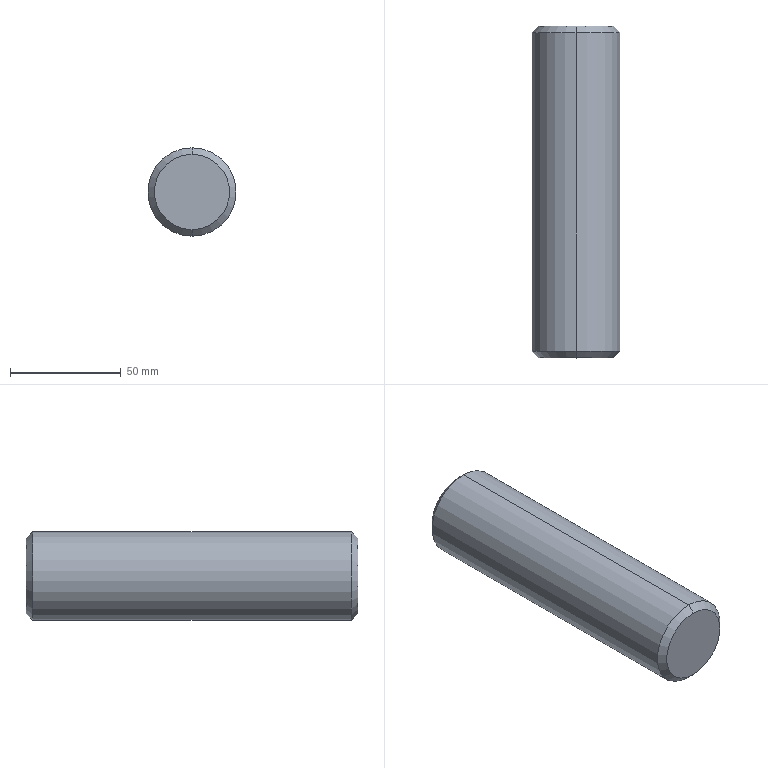Part | SolidWorks | 1 solid | 8 faces | box 40 x 150 x 40 mm | volume 187421 mm3 | cone 4 | cylinder 2 | plane 2 | commonest cylinder face diameters 40 x2
STEP:
#1=CARTESIAN_POINT('',(0.,0.,-17.));
#2=VERTEX_POINT('',#1);
#3=CARTESIAN_POINT('',(0.,0.,17.));
#4=VERTEX_POINT('',#3);
#5=CARTESIAN_POINT('',(0.,0.,0.));
#6=DIRECTION('',(0.,-1.,0.));
#7=DIRECTION('',(0.,0.,-1.));
#8=AXIS2_PLACEMENT_3D('',#5,#6,#7);
#9=CIRCLE('',#8,17.);
#10=EDGE_CURVE('',#2,#4,#9,.T.);
#11=ORIENTED_EDGE('',*,*,#10,.F.);
#12=CARTESIAN_POINT('',(0.,3.,-20.));
#13=VERTEX_POINT('',#12);
#14=CARTESIAN_POINT('',(0.,0.,-17.));
#15=DIRECTION('',(0.,0.7071,-0.7071));
#16=VECTOR('',#15,1000.);
#17=LINE('',#14,#16);
#18=EDGE_CURVE('',#2,#13,#17,.T.);
#19=ORIENTED_EDGE('',*,*,#18,.T.);
#20=CARTESIAN_POINT('',(0.,3.,20.));
#21=VERTEX_POINT('',#20);
#22=CARTESIAN_POINT('',(0.,3.,0.));
#23=DIRECTION('',(0.,-1.,0.));
#24=DIRECTION('',(0.,0.,-1.));
#25=AXIS2_PLACEMENT_3D('',#22,#23,#24);
#26=CIRCLE('',#25,20.);
#27=EDGE_CURVE('',#13,#21,#26,.T.);
#28=ORIENTED_EDGE('',*,*,#27,.T.);
#29=CARTESIAN_POINT('',(0.,0.,17.));
#30=DIRECTION('',(0.,0.7071,0.7071));
#31=VECTOR('',#30,1000.);
#32=LINE('',#29,#31);
#33=EDGE_CURVE('',#4,#21,#32,.T.);
#34=ORIENTED_EDGE('',*,*,#33,.F.);
#35=EDGE_LOOP('',(#11,#19,#28,#34));
#36=FACE_OUTER_BOUND('',#35,.T.);
#37=CARTESIAN_POINT('',(0.,0.,0.));
#38=DIRECTION('',(0.,1.,0.));
#39=DIRECTION('',(0.,0.,1.));
#40=AXIS2_PLACEMENT_3D('',#37,#38,#39);
#41=CONICAL_SURFACE('',#40,17.,0.7854);
#42=ADVANCED_FACE('',(#36),#41,.T.);
#43=CARTESIAN_POINT('',(0.,147.,-20.));
#44=VERTEX_POINT('',#43);
#45=CARTESIAN_POINT('',(0.,147.,20.));
#46=VERTEX_POINT('',#45);
#47=CARTESIAN_POINT('',(0.,147.,0.));
#48=DIRECTION('',(0.,-1.,0.));
#49=DIRECTION('',(0.,0.,-1.));
#50=AXIS2_PLACEMENT_3D('',#47,#48,#49);
#51=CIRCLE('',#50,20.);
#52=EDGE_CURVE('',#44,#46,#51,.T.);
#53=ORIENTED_EDGE('',*,*,#52,.T.);
#54=CARTESIAN_POINT('',(0.,0.,20.));
#55=DIRECTION('',(0.,-1.,0.));
#56=VECTOR('',#55,1000.);
#57=LINE('',#54,#56);
#58=EDGE_CURVE('',#46,#21,#57,.T.);
#59=ORIENTED_EDGE('',*,*,#58,.T.);
#60=ORIENTED_EDGE('',*,*,#27,.F.);
#61=CARTESIAN_POINT('',(0.,0.,-20.));
#62=DIRECTION('',(0.,-1.,0.));
#63=VECTOR('',#62,1000.);
#64=LINE('',#61,#63);
#65=EDGE_CURVE('',#44,#13,#64,.T.);
#66=ORIENTED_EDGE('',*,*,#65,.F.);
#67=EDGE_LOOP('',(#53,#59,#60,#66));
#68=FACE_OUTER_BOUND('',#67,.T.);
#69=CARTESIAN_POINT('',(0.,0.,0.));
#70=DIRECTION('',(0.,-1.,0.));
#71=DIRECTION('',(0.,0.,-1.));
#72=AXIS2_PLACEMENT_3D('',#69,#70,#71);
#73=CYLINDRICAL_SURFACE('',#72,20.);
#74=ADVANCED_FACE('',(#68),#73,.T.);
#75=CARTESIAN_POINT('',(0.,150.,-17.));
#76=VERTEX_POINT('',#75);
#77=CARTESIAN_POINT('',(0.,150.,17.));
#78=VERTEX_POINT('',#77);
#79=CARTESIAN_POINT('',(0.,150.,0.));
#80=DIRECTION('',(0.,-1.,0.));
#81=DIRECTION('',(0.,0.,-1.));
#82=AXIS2_PLACEMENT_3D('',#79,#80,#81);
#83=CIRCLE('',#82,17.);
#84=EDGE_CURVE('',#76,#78,#83,.T.);
#85=ORIENTED_EDGE('',*,*,#84,.T.);
#86=CARTESIAN_POINT('',(0.,147.,20.));
#87=DIRECTION('',(0.,-0.7071,0.7071));
#88=VECTOR('',#87,1000.);
#89=LINE('',#86,#88);
#90=EDGE_CURVE('',#78,#46,#89,.T.);
#91=ORIENTED_EDGE('',*,*,#90,.T.);
#92=ORIENTED_EDGE('',*,*,#52,.F.);
#93=CARTESIAN_POINT('',(0.,147.,-20.));
#94=DIRECTION('',(0.,-0.7071,-0.7071));
#95=VECTOR('',#94,1000.);
#96=LINE('',#93,#95);
#97=EDGE_CURVE('',#76,#44,#96,.T.);
#98=ORIENTED_EDGE('',*,*,#97,.F.);
#99=EDGE_LOOP('',(#85,#91,#92,#98));
#100=FACE_OUTER_BOUND('',#99,.T.);
#101=CARTESIAN_POINT('',(0.,147.,0.));
#102=DIRECTION('',(0.,-1.,0.));
#103=DIRECTION('',(0.,0.,-1.));
#104=AXIS2_PLACEMENT_3D('',#101,#102,#103);
#105=CONICAL_SURFACE('',#104,20.,0.7854);
#106=ADVANCED_FACE('',(#100),#105,.T.);
#107=ORIENTED_EDGE('',*,*,#84,.F.);
#108=CARTESIAN_POINT('',(0.,150.,0.));
#109=DIRECTION('',(0.,-1.,0.));
#110=DIRECTION('',(0.,0.,-1.));
#111=AXIS2_PLACEMENT_3D('',#108,#109,#110);
#112=CIRCLE('',#111,17.);
#113=EDGE_CURVE('',#78,#76,#112,.T.);
#114=ORIENTED_EDGE('',*,*,#113,.F.);
#115=EDGE_LOOP('',(#107,#114));
#116=FACE_OUTER_BOUND('',#115,.T.);
#117=CARTESIAN_POINT('',(0.,150.,0.));
#118=DIRECTION('',(0.,1.,0.));
#119=DIRECTION('',(0.,0.,1.));
#120=AXIS2_PLACEMENT_3D('',#117,#118,#119);
#121=PLANE('',#120);
#122=ADVANCED_FACE('',(#116),#121,.T.);
#123=ORIENTED_EDGE('',*,*,#90,.F.);
#124=ORIENTED_EDGE('',*,*,#113,.T.);
#125=ORIENTED_EDGE('',*,*,#97,.T.);
#126=CARTESIAN_POINT('',(0.,147.,0.));
#127=DIRECTION('',(0.,-1.,0.));
#128=DIRECTION('',(0.,0.,-1.));
#129=AXIS2_PLACEMENT_3D('',#126,#127,#128);
#130=CIRCLE('',#129,20.);
#131=EDGE_CURVE('',#46,#44,#130,.T.);
#132=ORIENTED_EDGE('',*,*,#131,.F.);
#133=EDGE_LOOP('',(#123,#124,#125,#132));
#134=FACE_OUTER_BOUND('',#133,.T.);
#135=CARTESIAN_POINT('',(0.,147.,0.));
#136=DIRECTION('',(0.,-1.,0.));
#137=DIRECTION('',(0.,0.,-1.));
#138=AXIS2_PLACEMENT_3D('',#135,#136,#137);
#139=CONICAL_SURFACE('',#138,20.,0.7854);
#140=ADVANCED_FACE('',(#134),#139,.T.);
#141=ORIENTED_EDGE('',*,*,#58,.F.);
#142=ORIENTED_EDGE('',*,*,#131,.T.);
#143=ORIENTED_EDGE('',*,*,#65,.T.);
#144=CARTESIAN_POINT('',(0.,3.,0.));
#145=DIRECTION('',(0.,-1.,0.));
#146=DIRECTION('',(0.,0.,-1.));
#147=AXIS2_PLACEMENT_3D('',#144,#145,#146);
#148=CIRCLE('',#147,20.);
#149=EDGE_CURVE('',#21,#13,#148,.T.);
#150=ORIENTED_EDGE('',*,*,#149,.F.);
#151=EDGE_LOOP('',(#141,#142,#143,#150));
#152=FACE_OUTER_BOUND('',#151,.T.);
#153=CARTESIAN_POINT('',(0.,0.,0.));
#154=DIRECTION('',(0.,-1.,0.));
#155=DIRECTION('',(0.,0.,-1.));
#156=AXIS2_PLACEMENT_3D('',#153,#154,#155);
#157=CYLINDRICAL_SURFACE('',#156,20.);
#158=ADVANCED_FACE('',(#152),#157,.T.);
#159=ORIENTED_EDGE('',*,*,#18,.F.);
#160=CARTESIAN_POINT('',(0.,0.,0.));
#161=DIRECTION('',(0.,-1.,0.));
#162=DIRECTION('',(0.,0.,-1.));
#163=AXIS2_PLACEMENT_3D('',#160,#161,#162);
#164=CIRCLE('',#163,17.);
#165=EDGE_CURVE('',#4,#2,#164,.T.);
#166=ORIENTED_EDGE('',*,*,#165,.F.);
#167=ORIENTED_EDGE('',*,*,#33,.T.);
#168=ORIENTED_EDGE('',*,*,#149,.T.);
#169=EDGE_LOOP('',(#159,#166,#167,#168));
#170=FACE_OUTER_BOUND('',#169,.T.);
#171=CARTESIAN_POINT('',(0.,0.,0.));
#172=DIRECTION('',(0.,1.,0.));
#173=DIRECTION('',(0.,0.,1.));
#174=AXIS2_PLACEMENT_3D('',#171,#172,#173);
#175=CONICAL_SURFACE('',#174,17.,0.7854);
#176=ADVANCED_FACE('',(#170),#175,.T.);
#177=ORIENTED_EDGE('',*,*,#165,.T.);
#178=ORIENTED_EDGE('',*,*,#10,.T.);
#179=EDGE_LOOP('',(#177,#178));
#180=FACE_OUTER_BOUND('',#179,.T.);
#181=CARTESIAN_POINT('',(0.,0.,0.));
#182=DIRECTION('',(0.,-1.,0.));
#183=DIRECTION('',(0.,0.,-1.));
#184=AXIS2_PLACEMENT_3D('',#181,#182,#183);
#185=PLANE('',#184);
#186=ADVANCED_FACE('',(#180),#185,.T.);
#187=CLOSED_SHELL('',(#42,#74,#106,#122,#140,#158,#176,#186));
#188=MANIFOLD_SOLID_BREP('',#187);
#189=CARTESIAN_POINT('',(0.,0.,0.));
#190=DIRECTION('',(0.,0.,1.));
#191=DIRECTION('',(1.,0.,0.));
#192=AXIS2_PLACEMENT_3D('',#189,#190,#191);
#193=(LENGTH_UNIT()NAMED_UNIT(*)SI_UNIT(.MILLI.,.METRE.));
#194=UNCERTAINTY_MEASURE_WITH_UNIT(LENGTH_MEASURE(0.00001),#193,'','');
#195=(NAMED_UNIT(*)PLANE_ANGLE_UNIT()SI_UNIT($,.RADIAN.));
#196=(NAMED_UNIT(*)SI_UNIT($,.STERADIAN.)SOLID_ANGLE_UNIT());
#197=(GEOMETRIC_REPRESENTATION_CONTEXT(3)GLOBAL_UNCERTAINTY_ASSIGNED_CONTEXT((#194))GLOBAL_UNIT_ASSIGNED_CONTEXT((#193,#195,#196))REPRESENTATION_CONTEXT('',''));
#198=ADVANCED_BREP_SHAPE_REPRESENTATION('',(#188,#192),#197);